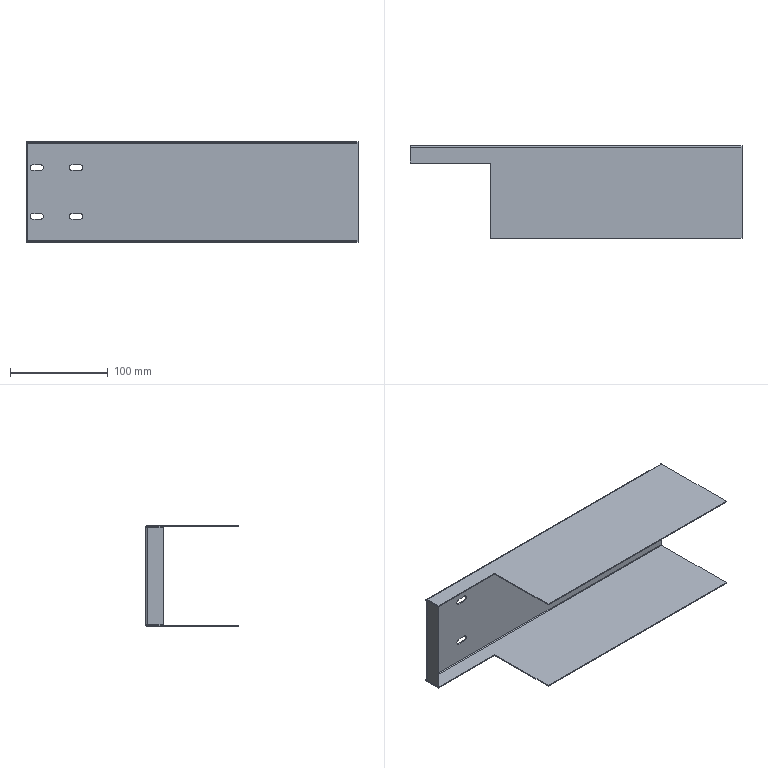Part | SolidWorks | features EdgeFlange 1, Extrusion 1, FlatPattern 1, HoleWzd 1, ICE 1, SheetMetal 1, SolidToSheetMetal 1 | 1 solid | 52 faces | box 340 x 95 x 103 mm | volume 87299 mm3 | plane 38 | cylinder 14 | commonest cylinder face diameters 5.8 x8 1.473 x3 3.473 x3
STEP:
#1=CARTESIAN_POINT('',(-163.,47.5,-27.9));
#2=VERTEX_POINT('',#1);
#3=CARTESIAN_POINT('',(-163.,47.5,-22.1));
#4=VERTEX_POINT('',#3);
#5=CARTESIAN_POINT('',(-163.,47.5,-25.));
#6=DIRECTION('',(0.,1.,0.));
#7=DIRECTION('',(0.,0.,1.));
#8=AXIS2_PLACEMENT_3D('',#5,#6,#7);
#9=CIRCLE('',#8,2.9);
#10=EDGE_CURVE('',#2,#4,#9,.T.);
#11=ORIENTED_EDGE('',*,*,#10,.F.);
#12=CARTESIAN_POINT('',(-155.,47.5,-27.9));
#13=VERTEX_POINT('',#12);
#14=CARTESIAN_POINT('',(-163.,47.5,-27.9));
#15=DIRECTION('',(1.,0.,0.));
#16=VECTOR('',#15,1000.);
#17=LINE('',#14,#16);
#18=EDGE_CURVE('',#2,#13,#17,.T.);
#19=ORIENTED_EDGE('',*,*,#18,.T.);
#20=CARTESIAN_POINT('',(-155.,47.5,-22.1));
#21=VERTEX_POINT('',#20);
#22=CARTESIAN_POINT('',(-155.,47.5,-25.));
#23=DIRECTION('',(0.,1.,0.));
#24=DIRECTION('',(0.,0.,1.));
#25=AXIS2_PLACEMENT_3D('',#22,#23,#24);
#26=CIRCLE('',#25,2.9);
#27=EDGE_CURVE('',#21,#13,#26,.T.);
#28=ORIENTED_EDGE('',*,*,#27,.F.);
#29=CARTESIAN_POINT('',(-163.,47.5,-22.1));
#30=DIRECTION('',(1.,0.,0.));
#31=VECTOR('',#30,1000.);
#32=LINE('',#29,#31);
#33=EDGE_CURVE('',#4,#21,#32,.T.);
#34=ORIENTED_EDGE('',*,*,#33,.F.);
#35=EDGE_LOOP('',(#11,#19,#28,#34));
#36=FACE_BOUND('',#35,.T.);
#37=CARTESIAN_POINT('',(-123.,47.5,-27.9));
#38=VERTEX_POINT('',#37);
#39=CARTESIAN_POINT('',(-123.,47.5,-22.1));
#40=VERTEX_POINT('',#39);
#41=CARTESIAN_POINT('',(-123.,47.5,-25.));
#42=DIRECTION('',(0.,1.,0.));
#43=DIRECTION('',(0.,0.,1.));
#44=AXIS2_PLACEMENT_3D('',#41,#42,#43);
#45=CIRCLE('',#44,2.9);
#46=EDGE_CURVE('',#38,#40,#45,.T.);
#47=ORIENTED_EDGE('',*,*,#46,.F.);
#48=CARTESIAN_POINT('',(-115.,47.5,-27.9));
#49=VERTEX_POINT('',#48);
#50=CARTESIAN_POINT('',(-123.,47.5,-27.9));
#51=DIRECTION('',(1.,0.,0.));
#52=VECTOR('',#51,1000.);
#53=LINE('',#50,#52);
#54=EDGE_CURVE('',#38,#49,#53,.T.);
#55=ORIENTED_EDGE('',*,*,#54,.T.);
#56=CARTESIAN_POINT('',(-115.,47.5,-22.1));
#57=VERTEX_POINT('',#56);
#58=CARTESIAN_POINT('',(-115.,47.5,-25.));
#59=DIRECTION('',(0.,1.,0.));
#60=DIRECTION('',(0.,0.,1.));
#61=AXIS2_PLACEMENT_3D('',#58,#59,#60);
#62=CIRCLE('',#61,2.9);
#63=EDGE_CURVE('',#57,#49,#62,.T.);
#64=ORIENTED_EDGE('',*,*,#63,.F.);
#65=CARTESIAN_POINT('',(-123.,47.5,-22.1));
#66=DIRECTION('',(1.,0.,0.));
#67=VECTOR('',#66,1000.);
#68=LINE('',#65,#67);
#69=EDGE_CURVE('',#40,#57,#68,.T.);
#70=ORIENTED_EDGE('',*,*,#69,.F.);
#71=EDGE_LOOP('',(#47,#55,#64,#70));
#72=FACE_BOUND('',#71,.T.);
#73=CARTESIAN_POINT('',(-168.263,47.5,-49.763));
#74=VERTEX_POINT('',#73);
#75=CARTESIAN_POINT('',(-168.263,47.5,49.763));
#76=VERTEX_POINT('',#75);
#77=CARTESIAN_POINT('',(-168.263,47.5,-49.763));
#78=DIRECTION('',(0.,0.,1.));
#79=VECTOR('',#78,1000.);
#80=LINE('',#77,#79);
#81=EDGE_CURVE('',#74,#76,#80,.T.);
#82=ORIENTED_EDGE('',*,*,#81,.T.);
#83=CARTESIAN_POINT('',(170.,47.5,49.763));
#84=VERTEX_POINT('',#83);
#85=CARTESIAN_POINT('',(-170.,47.5,49.763));
#86=DIRECTION('',(1.,0.,0.));
#87=VECTOR('',#86,1000.);
#88=LINE('',#85,#87);
#89=EDGE_CURVE('',#76,#84,#88,.T.);
#90=ORIENTED_EDGE('',*,*,#89,.T.);
#91=CARTESIAN_POINT('',(170.,47.5,-49.763));
#92=VERTEX_POINT('',#91);
#93=CARTESIAN_POINT('',(170.,47.5,51.5));
#94=DIRECTION('',(0.,0.,-1.));
#95=VECTOR('',#94,1000.);
#96=LINE('',#93,#95);
#97=EDGE_CURVE('',#84,#92,#96,.T.);
#98=ORIENTED_EDGE('',*,*,#97,.T.);
#99=CARTESIAN_POINT('',(-170.,47.5,-49.763));
#100=DIRECTION('',(-1.,0.,0.));
#101=VECTOR('',#100,1000.);
#102=LINE('',#99,#101);
#103=EDGE_CURVE('',#92,#74,#102,.T.);
#104=ORIENTED_EDGE('',*,*,#103,.T.);
#105=EDGE_LOOP('',(#82,#90,#98,#104));
#106=FACE_OUTER_BOUND('',#105,.T.);
#107=CARTESIAN_POINT('',(-123.,47.5,22.1));
#108=VERTEX_POINT('',#107);
#109=CARTESIAN_POINT('',(-123.,47.5,27.9));
#110=VERTEX_POINT('',#109);
#111=CARTESIAN_POINT('',(-123.,47.5,25.));
#112=DIRECTION('',(0.,1.,0.));
#113=DIRECTION('',(0.,0.,1.));
#114=AXIS2_PLACEMENT_3D('',#111,#112,#113);
#115=CIRCLE('',#114,2.9);
#116=EDGE_CURVE('',#108,#110,#115,.T.);
#117=ORIENTED_EDGE('',*,*,#116,.F.);
#118=CARTESIAN_POINT('',(-115.,47.5,22.1));
#119=VERTEX_POINT('',#118);
#120=CARTESIAN_POINT('',(-123.,47.5,22.1));
#121=DIRECTION('',(1.,0.,0.));
#122=VECTOR('',#121,1000.);
#123=LINE('',#120,#122);
#124=EDGE_CURVE('',#108,#119,#123,.T.);
#125=ORIENTED_EDGE('',*,*,#124,.T.);
#126=CARTESIAN_POINT('',(-115.,47.5,27.9));
#127=VERTEX_POINT('',#126);
#128=CARTESIAN_POINT('',(-115.,47.5,25.));
#129=DIRECTION('',(0.,1.,0.));
#130=DIRECTION('',(0.,0.,1.));
#131=AXIS2_PLACEMENT_3D('',#128,#129,#130);
#132=CIRCLE('',#131,2.9);
#133=EDGE_CURVE('',#127,#119,#132,.T.);
#134=ORIENTED_EDGE('',*,*,#133,.F.);
#135=CARTESIAN_POINT('',(-123.,47.5,27.9));
#136=DIRECTION('',(1.,0.,0.));
#137=VECTOR('',#136,1000.);
#138=LINE('',#135,#137);
#139=EDGE_CURVE('',#110,#127,#138,.T.);
#140=ORIENTED_EDGE('',*,*,#139,.F.);
#141=EDGE_LOOP('',(#117,#125,#134,#140));
#142=FACE_BOUND('',#141,.T.);
#143=CARTESIAN_POINT('',(-163.,47.5,27.9));
#144=VERTEX_POINT('',#143);
#145=CARTESIAN_POINT('',(-155.,47.5,27.9));
#146=VERTEX_POINT('',#145);
#147=CARTESIAN_POINT('',(-163.,47.5,27.9));
#148=DIRECTION('',(1.,0.,0.));
#149=VECTOR('',#148,1000.);
#150=LINE('',#147,#149);
#151=EDGE_CURVE('',#144,#146,#150,.T.);
#152=ORIENTED_EDGE('',*,*,#151,.F.);
#153=CARTESIAN_POINT('',(-163.,47.5,22.1));
#154=VERTEX_POINT('',#153);
#155=CARTESIAN_POINT('',(-163.,47.5,25.));
#156=DIRECTION('',(0.,1.,0.));
#157=DIRECTION('',(0.,0.,1.));
#158=AXIS2_PLACEMENT_3D('',#155,#156,#157);
#159=CIRCLE('',#158,2.9);
#160=EDGE_CURVE('',#154,#144,#159,.T.);
#161=ORIENTED_EDGE('',*,*,#160,.F.);
#162=CARTESIAN_POINT('',(-155.,47.5,22.1));
#163=VERTEX_POINT('',#162);
#164=CARTESIAN_POINT('',(-163.,47.5,22.1));
#165=DIRECTION('',(1.,0.,0.));
#166=VECTOR('',#165,1000.);
#167=LINE('',#164,#166);
#168=EDGE_CURVE('',#154,#163,#167,.T.);
#169=ORIENTED_EDGE('',*,*,#168,.T.);
#170=CARTESIAN_POINT('',(-155.,47.5,25.));
#171=DIRECTION('',(0.,1.,0.));
#172=DIRECTION('',(0.,0.,1.));
#173=AXIS2_PLACEMENT_3D('',#170,#171,#172);
#174=CIRCLE('',#173,2.9);
#175=EDGE_CURVE('',#146,#163,#174,.T.);
#176=ORIENTED_EDGE('',*,*,#175,.F.);
#177=EDGE_LOOP('',(#152,#161,#169,#176));
#178=FACE_BOUND('',#177,.T.);
#179=CARTESIAN_POINT('',(-170.,47.5,51.5));
#180=DIRECTION('',(0.,-1.,0.));
#181=DIRECTION('',(0.,0.,-1.));
#182=AXIS2_PLACEMENT_3D('',#179,#180,#181);
#183=PLANE('',#182);
#184=ADVANCED_FACE('',(#36,#72,#106,#142,#178),#183,.F.);
#185=CARTESIAN_POINT('',(-170.,47.5,49.763));
#186=VERTEX_POINT('',#185);
#187=CARTESIAN_POINT('',(-170.,47.5,49.763));
#188=DIRECTION('',(1.,0.,0.));
#189=VECTOR('',#188,1000.);
#190=LINE('',#187,#189);
#191=EDGE_CURVE('',#186,#76,#190,.T.);
#192=ORIENTED_EDGE('',*,*,#191,.T.);
#193=CARTESIAN_POINT('',(-169.836,46.5,49.763));
#194=VERTEX_POINT('',#193);
#195=CARTESIAN_POINT('',(-168.263,45.763,49.763));
#196=DIRECTION('',(0.,0.,1.));
#197=DIRECTION('',(-1.,0.,0.));
#198=AXIS2_PLACEMENT_3D('',#195,#196,#197);
#199=CIRCLE('',#198,1.737);
#200=EDGE_CURVE('',#76,#194,#199,.T.);
#201=ORIENTED_EDGE('',*,*,#200,.T.);
#202=CARTESIAN_POINT('',(-170.,46.5,49.763));
#203=VERTEX_POINT('',#202);
#204=CARTESIAN_POINT('',(-170.,46.5,49.763));
#205=DIRECTION('',(1.,0.,0.));
#206=VECTOR('',#205,1000.);
#207=LINE('',#204,#206);
#208=EDGE_CURVE('',#203,#194,#207,.T.);
#209=ORIENTED_EDGE('',*,*,#208,.F.);
#210=CARTESIAN_POINT('',(-170.,47.5,49.763));
#211=DIRECTION('',(0.,1.,0.));
#212=VECTOR('',#211,1000.);
#213=LINE('',#210,#212);
#214=EDGE_CURVE('',#203,#186,#213,.T.);
#215=ORIENTED_EDGE('',*,*,#214,.T.);
#216=EDGE_LOOP('',(#192,#201,#209,#215));
#217=FACE_OUTER_BOUND('',#216,.T.);
#218=CARTESIAN_POINT('',(-168.263,46.5,49.763));
#219=DIRECTION('',(0.,0.,-1.));
#220=DIRECTION('',(0.,1.,0.));
#221=AXIS2_PLACEMENT_3D('',#218,#219,#220);
#222=PLANE('',#221);
#223=ADVANCED_FACE('',(#217),#222,.T.);
#224=CARTESIAN_POINT('',(-170.,46.5,-49.763));
#225=VERTEX_POINT('',#224);
#226=CARTESIAN_POINT('',(-169.836,46.5,-49.763));
#227=VERTEX_POINT('',#226);
#228=CARTESIAN_POINT('',(-170.,46.5,-49.763));
#229=DIRECTION('',(1.,0.,0.));
#230=VECTOR('',#229,1000.);
#231=LINE('',#228,#230);
#232=EDGE_CURVE('',#225,#227,#231,.T.);
#233=ORIENTED_EDGE('',*,*,#232,.T.);
#234=CARTESIAN_POINT('',(-168.263,45.763,-49.763));
#235=DIRECTION('',(0.,0.,-1.));
#236=DIRECTION('',(-1.,0.,0.));
#237=AXIS2_PLACEMENT_3D('',#234,#235,#236);
#238=CIRCLE('',#237,1.737);
#239=EDGE_CURVE('',#227,#74,#238,.T.);
#240=ORIENTED_EDGE('',*,*,#239,.T.);
#241=CARTESIAN_POINT('',(-170.,47.5,-49.763));
#242=VERTEX_POINT('',#241);
#243=CARTESIAN_POINT('',(-170.,47.5,-49.763));
#244=DIRECTION('',(1.,0.,0.));
#245=VECTOR('',#244,1000.);
#246=LINE('',#243,#245);
#247=EDGE_CURVE('',#242,#74,#246,.T.);
#248=ORIENTED_EDGE('',*,*,#247,.F.);
#249=CARTESIAN_POINT('',(-170.,47.5,-49.763));
#250=DIRECTION('',(0.,1.,0.));
#251=VECTOR('',#250,1000.);
#252=LINE('',#249,#251);
#253=EDGE_CURVE('',#225,#242,#252,.T.);
#254=ORIENTED_EDGE('',*,*,#253,.F.);
#255=EDGE_LOOP('',(#233,#240,#248,#254));
#256=FACE_OUTER_BOUND('',#255,.T.);
#257=CARTESIAN_POINT('',(-170.,46.5,-49.763));
#258=DIRECTION('',(0.,0.,1.));
#259=DIRECTION('',(1.,0.,0.));
#260=AXIS2_PLACEMENT_3D('',#257,#258,#259);
#261=PLANE('',#260);
#262=ADVANCED_FACE('',(#256),#261,.T.);
#263=CARTESIAN_POINT('',(-163.,46.5,-27.9));
#264=VERTEX_POINT('',#263);
#265=CARTESIAN_POINT('',(-155.,46.5,-27.9));
#266=VERTEX_POINT('',#265);
#267=CARTESIAN_POINT('',(-170.,46.5,-27.9));
#268=DIRECTION('',(1.,0.,0.));
#269=VECTOR('',#268,1000.);
#270=LINE('',#267,#269);
#271=EDGE_CURVE('',#264,#266,#270,.T.);
#272=ORIENTED_EDGE('',*,*,#271,.F.);
#273=CARTESIAN_POINT('',(-163.,46.5,-22.1));
#274=VERTEX_POINT('',#273);
#275=CARTESIAN_POINT('',(-163.,46.5,-25.));
#276=DIRECTION('',(0.,-1.,0.));
#277=DIRECTION('',(0.,0.,-1.));
#278=AXIS2_PLACEMENT_3D('',#275,#276,#277);
#279=CIRCLE('',#278,2.9);
#280=EDGE_CURVE('',#274,#264,#279,.T.);
#281=ORIENTED_EDGE('',*,*,#280,.F.);
#282=CARTESIAN_POINT('',(-155.,46.5,-22.1));
#283=VERTEX_POINT('',#282);
#284=CARTESIAN_POINT('',(-170.,46.5,-22.1));
#285=DIRECTION('',(-1.,0.,0.));
#286=VECTOR('',#285,1000.);
#287=LINE('',#284,#286);
#288=EDGE_CURVE('',#283,#274,#287,.T.);
#289=ORIENTED_EDGE('',*,*,#288,.F.);
#290=CARTESIAN_POINT('',(-155.,46.5,-25.));
#291=DIRECTION('',(0.,-1.,0.));
#292=DIRECTION('',(0.,0.,-1.));
#293=AXIS2_PLACEMENT_3D('',#290,#291,#292);
#294=CIRCLE('',#293,2.9);
#295=EDGE_CURVE('',#266,#283,#294,.T.);
#296=ORIENTED_EDGE('',*,*,#295,.F.);
#297=EDGE_LOOP('',(#272,#281,#289,#296));
#298=FACE_BOUND('',#297,.T.);
#299=CARTESIAN_POINT('',(-123.,46.5,-27.9));
#300=VERTEX_POINT('',#299);
#301=CARTESIAN_POINT('',(-115.,46.5,-27.9));
#302=VERTEX_POINT('',#301);
#303=CARTESIAN_POINT('',(-170.,46.5,-27.9));
#304=DIRECTION('',(1.,0.,0.));
#305=VECTOR('',#304,1000.);
#306=LINE('',#303,#305);
#307=EDGE_CURVE('',#300,#302,#306,.T.);
#308=ORIENTED_EDGE('',*,*,#307,.F.);
#309=CARTESIAN_POINT('',(-123.,46.5,-22.1));
#310=VERTEX_POINT('',#309);
#311=CARTESIAN_POINT('',(-123.,46.5,-25.));
#312=DIRECTION('',(0.,-1.,0.));
#313=DIRECTION('',(0.,0.,-1.));
#314=AXIS2_PLACEMENT_3D('',#311,#312,#313);
#315=CIRCLE('',#314,2.9);
#316=EDGE_CURVE('',#310,#300,#315,.T.);
#317=ORIENTED_EDGE('',*,*,#316,.F.);
#318=CARTESIAN_POINT('',(-115.,46.5,-22.1));
#319=VERTEX_POINT('',#318);
#320=CARTESIAN_POINT('',(-170.,46.5,-22.1));
#321=DIRECTION('',(-1.,0.,0.));
#322=VECTOR('',#321,1000.);
#323=LINE('',#320,#322);
#324=EDGE_CURVE('',#319,#310,#323,.T.);
#325=ORIENTED_EDGE('',*,*,#324,.F.);
#326=CARTESIAN_POINT('',(-115.,46.5,-25.));
#327=DIRECTION('',(0.,-1.,0.));
#328=DIRECTION('',(0.,0.,-1.));
#329=AXIS2_PLACEMENT_3D('',#326,#327,#328);
#330=CIRCLE('',#329,2.9);
#331=EDGE_CURVE('',#302,#319,#330,.T.);
#332=ORIENTED_EDGE('',*,*,#331,.F.);
#333=EDGE_LOOP('',(#308,#317,#325,#332));
#334=FACE_BOUND('',#333,.T.);
#335=CARTESIAN_POINT('',(-155.,46.5,22.1));
#336=VERTEX_POINT('',#335);
#337=CARTESIAN_POINT('',(-155.,46.5,27.9));
#338=VERTEX_POINT('',#337);
#339=CARTESIAN_POINT('',(-155.,46.5,25.));
#340=DIRECTION('',(0.,-1.,0.));
#341=DIRECTION('',(0.,0.,-1.));
#342=AXIS2_PLACEMENT_3D('',#339,#340,#341);
#343=CIRCLE('',#342,2.9);
#344=EDGE_CURVE('',#336,#338,#343,.T.);
#345=ORIENTED_EDGE('',*,*,#344,.F.);
#346=CARTESIAN_POINT('',(-163.,46.5,22.1));
#347=VERTEX_POINT('',#346);
#348=CARTESIAN_POINT('',(-170.,46.5,22.1));
#349=DIRECTION('',(1.,0.,0.));
#350=VECTOR('',#349,1000.);
#351=LINE('',#348,#350);
#352=EDGE_CURVE('',#347,#336,#351,.T.);
#353=ORIENTED_EDGE('',*,*,#352,.F.);
#354=CARTESIAN_POINT('',(-163.,46.5,27.9));
#355=VERTEX_POINT('',#354);
#356=CARTESIAN_POINT('',(-163.,46.5,25.));
#357=DIRECTION('',(0.,-1.,0.));
#358=DIRECTION('',(0.,0.,-1.));
#359=AXIS2_PLACEMENT_3D('',#356,#357,#358);
#360=CIRCLE('',#359,2.9);
#361=EDGE_CURVE('',#355,#347,#360,.T.);
#362=ORIENTED_EDGE('',*,*,#361,.F.);
#363=CARTESIAN_POINT('',(-170.,46.5,27.9));
#364=DIRECTION('',(-1.,0.,0.));
#365=VECTOR('',#364,1000.);
#366=LINE('',#363,#365);
#367=EDGE_CURVE('',#338,#355,#366,.T.);
#368=ORIENTED_EDGE('',*,*,#367,.F.);
#369=EDGE_LOOP('',(#345,#353,#362,#368));
#370=FACE_BOUND('',#369,.T.);
#371=CARTESIAN_POINT('',(-123.,46.5,22.1));
#372=VERTEX_POINT('',#371);
#373=CARTESIAN_POINT('',(-115.,46.5,22.1));
#374=VERTEX_POINT('',#373);
#375=CARTESIAN_POINT('',(-170.,46.5,22.1));
#376=DIRECTION('',(1.,0.,0.));
#377=VECTOR('',#376,1000.);
#378=LINE('',#375,#377);
#379=EDGE_CURVE('',#372,#374,#378,.T.);
#380=ORIENTED_EDGE('',*,*,#379,.F.);
#381=CARTESIAN_POINT('',(-123.,46.5,27.9));
#382=VERTEX_POINT('',#381);
#383=CARTESIAN_POINT('',(-123.,46.5,25.));
#384=DIRECTION('',(0.,-1.,0.));
#385=DIRECTION('',(0.,0.,-1.));
#386=AXIS2_PLACEMENT_3D('',#383,#384,#385);
#387=CIRCLE('',#386,2.9);
#388=EDGE_CURVE('',#382,#372,#387,.T.);
#389=ORIENTED_EDGE('',*,*,#388,.F.);
#390=CARTESIAN_POINT('',(-115.,46.5,27.9));
#391=VERTEX_POINT('',#390);
#392=CARTESIAN_POINT('',(-170.,46.5,27.9));
#393=DIRECTION('',(-1.,0.,0.));
#394=VECTOR('',#393,1000.);
#395=LINE('',#392,#394);
#396=EDGE_CURVE('',#391,#382,#395,.T.);
#397=ORIENTED_EDGE('',*,*,#396,.F.);
#398=CARTESIAN_POINT('',(-115.,46.5,25.));
#399=DIRECTION('',(0.,-1.,0.));
#400=DIRECTION('',(0.,0.,-1.));
#401=AXIS2_PLACEMENT_3D('',#398,#399,#400);
#402=CIRCLE('',#401,2.9);
#403=EDGE_CURVE('',#374,#391,#402,.T.);
#404=ORIENTED_EDGE('',*,*,#403,.F.);
#405=EDGE_LOOP('',(#380,#389,#397,#404));
#406=FACE_BOUND('',#405,.T.);
#407=CARTESIAN_POINT('',(-168.263,46.5,49.763));
#408=VERTEX_POINT('',#407);
#409=CARTESIAN_POINT('',(170.,46.5,49.763));
#410=VERTEX_POINT('',#409);
#411=CARTESIAN_POINT('',(-170.,46.5,49.763));
#412=DIRECTION('',(1.,0.,0.));
#413=VECTOR('',#412,1000.);
#414=LINE('',#411,#413);
#415=EDGE_CURVE('',#408,#410,#414,.T.);
#416=ORIENTED_EDGE('',*,*,#415,.F.);
#417=CARTESIAN_POINT('',(-168.263,46.5,-49.763));
#418=VERTEX_POINT('',#417);
#419=CARTESIAN_POINT('',(-168.263,46.5,-49.763));
#420=DIRECTION('',(0.,0.,1.));
#421=VECTOR('',#420,1000.);
#422=LINE('',#419,#421);
#423=EDGE_CURVE('',#418,#408,#422,.T.);
#424=ORIENTED_EDGE('',*,*,#423,.F.);
#425=CARTESIAN_POINT('',(170.,46.5,-49.763));
#426=VERTEX_POINT('',#425);
#427=CARTESIAN_POINT('',(-170.,46.5,-49.763));
#428=DIRECTION('',(-1.,0.,0.));
#429=VECTOR('',#428,1000.);
#430=LINE('',#427,#429);
#431=EDGE_CURVE('',#426,#418,#430,.T.);
#432=ORIENTED_EDGE('',*,*,#431,.F.);
#433=CARTESIAN_POINT('',(170.,46.5,51.5));
#434=DIRECTION('',(0.,0.,-1.));
#435=VECTOR('',#434,1000.);
#436=LINE('',#433,#435);
#437=EDGE_CURVE('',#410,#426,#436,.T.);
#438=ORIENTED_EDGE('',*,*,#437,.F.);
#439=EDGE_LOOP('',(#416,#424,#432,#438));
#440=FACE_OUTER_BOUND('',#439,.T.);
#441=CARTESIAN_POINT('',(-170.,46.5,51.5));
#442=DIRECTION('',(0.,-1.,0.));
#443=DIRECTION('',(0.,0.,-1.));
#444=AXIS2_PLACEMENT_3D('',#441,#442,#443);
#445=PLANE('',#444);
#446=ADVANCED_FACE('',(#298,#334,#370,#406,#440),#445,.T.);
#447=CARTESIAN_POINT('',(170.,47.5,49.763));
#448=DIRECTION('',(0.,1.,0.));
#449=VECTOR('',#448,1000.);
#450=LINE('',#447,#449);
#451=EDGE_CURVE('',#410,#84,#450,.T.);
#452=ORIENTED_EDGE('',*,*,#451,.F.);
#453=ORIENTED_EDGE('',*,*,#437,.T.);
#454=CARTESIAN_POINT('',(170.,47.5,-49.763));
#455=DIRECTION('',(0.,1.,0.));
#456=VECTOR('',#455,1000.);
#457=LINE('',#454,#456);
#458=EDGE_CURVE('',#426,#92,#457,.T.);
#459=ORIENTED_EDGE('',*,*,#458,.T.);
#460=ORIENTED_EDGE('',*,*,#97,.F.);
#461=EDGE_LOOP('',(#452,#453,#459,#460));
#462=FACE_OUTER_BOUND('',#461,.T.);
#463=CARTESIAN_POINT('',(170.,47.5,51.5));
#464=DIRECTION('',(-1.,0.,0.));
#465=DIRECTION('',(0.,0.,-1.));
#466=AXIS2_PLACEMENT_3D('',#463,#464,#465);
#467=PLANE('',#466);
#468=ADVANCED_FACE('',(#462),#467,.F.);
#469=ORIENTED_EDGE('',*,*,#458,.F.);
#470=CARTESIAN_POINT('',(170.,45.763,-50.5));
#471=VERTEX_POINT('',#470);
#472=CARTESIAN_POINT('',(170.,45.763,-49.763));
#473=DIRECTION('',(-1.,0.,0.));
#474=DIRECTION('',(0.,0.,-1.));
#475=AXIS2_PLACEMENT_3D('',#472,#473,#474);
#476=CIRCLE('',#475,0.7366);
#477=EDGE_CURVE('',#426,#471,#476,.T.);
#478=ORIENTED_EDGE('',*,*,#477,.T.);
#479=CARTESIAN_POINT('',(170.,45.763,-51.5));
#480=VERTEX_POINT('',#479);
#481=CARTESIAN_POINT('',(170.,45.763,-51.5));
#482=DIRECTION('',(0.,0.,-1.));
#483=VECTOR('',#482,1000.);
#484=LINE('',#481,#483);
#485=EDGE_CURVE('',#471,#480,#484,.T.);
#486=ORIENTED_EDGE('',*,*,#485,.T.);
#487=CARTESIAN_POINT('',(170.,45.763,-49.763));
#488=DIRECTION('',(-1.,0.,0.));
#489=DIRECTION('',(0.,0.,1.));
#490=AXIS2_PLACEMENT_3D('',#487,#488,#489);
#491=CIRCLE('',#490,1.737);
#492=EDGE_CURVE('',#92,#480,#491,.T.);
#493=ORIENTED_EDGE('',*,*,#492,.F.);
#494=EDGE_LOOP('',(#469,#478,#486,#493));
#495=FACE_OUTER_BOUND('',#494,.T.);
#496=CARTESIAN_POINT('',(170.,45.763,-49.763));
#497=DIRECTION('',(1.,0.,0.));
#498=DIRECTION('',(0.,0.,-1.));
#499=AXIS2_PLACEMENT_3D('',#496,#497,#498);
#500=PLANE('',#499);
#501=ADVANCED_FACE('',(#495),#500,.T.);
#502=ORIENTED_EDGE('',*,*,#485,.F.);
#503=CARTESIAN_POINT('',(170.,-47.5,-50.5));
#504=VERTEX_POINT('',#503);
#505=CARTESIAN_POINT('',(170.,0.,-50.5));
#506=DIRECTION('',(0.,1.,0.));
#507=VECTOR('',#506,1000.);
#508=LINE('',#505,#507);
#509=EDGE_CURVE('',#504,#471,#508,.T.);
#510=ORIENTED_EDGE('',*,*,#509,.F.);
#511=CARTESIAN_POINT('',(170.,-47.5,-51.5));
#512=VERTEX_POINT('',#511);
#513=CARTESIAN_POINT('',(170.,-47.5,-51.5));
#514=DIRECTION('',(0.,0.,-1.));
#515=VECTOR('',#514,1000.);
#516=LINE('',#513,#515);
#517=EDGE_CURVE('',#504,#512,#516,.T.);
#518=ORIENTED_EDGE('',*,*,#517,.T.);
#519=CARTESIAN_POINT('',(170.,-47.5,-51.5));
#520=DIRECTION('',(0.,1.,0.));
#521=VECTOR('',#520,1000.);
#522=LINE('',#519,#521);
#523=EDGE_CURVE('',#512,#480,#522,.T.);
#524=ORIENTED_EDGE('',*,*,#523,.T.);
#525=EDGE_LOOP('',(#502,#510,#518,#524));
#526=FACE_OUTER_BOUND('',#525,.T.);
#527=CARTESIAN_POINT('',(170.,-47.5,-51.5));
#528=DIRECTION('',(-1.,0.,0.));
#529=DIRECTION('',(0.,1.,0.));
#530=AXIS2_PLACEMENT_3D('',#527,#528,#529);
#531=PLANE('',#530);
#532=ADVANCED_FACE('',(#526),#531,.F.);
#533=CARTESIAN_POINT('',(-88.,-47.5,-50.5));
#534=VERTEX_POINT('',#533);
#535=CARTESIAN_POINT('',(-88.,-47.5,-51.5));
#536=VERTEX_POINT('',#535);
#537=CARTESIAN_POINT('',(-88.,-47.5,51.5));
#538=DIRECTION('',(0.,0.,-1.));
#539=VECTOR('',#538,1000.);
#540=LINE('',#537,#539);
#541=EDGE_CURVE('',#534,#536,#540,.T.);
#542=ORIENTED_EDGE('',*,*,#541,.T.);
#543=CARTESIAN_POINT('',(-170.,-47.5,-51.5));
#544=DIRECTION('',(1.,0.,0.));
#545=VECTOR('',#544,1000.);
#546=LINE('',#543,#545);
#547=EDGE_CURVE('',#536,#512,#546,.T.);
#548=ORIENTED_EDGE('',*,*,#547,.T.);
#549=ORIENTED_EDGE('',*,*,#517,.F.);
#550=CARTESIAN_POINT('',(0.,-47.5,-50.5));
#551=DIRECTION('',(1.,0.,0.));
#552=VECTOR('',#551,1000.);
#553=LINE('',#550,#552);
#554=EDGE_CURVE('',#534,#504,#553,.T.);
#555=ORIENTED_EDGE('',*,*,#554,.F.);
#556=EDGE_LOOP('',(#542,#548,#549,#555));
#557=FACE_OUTER_BOUND('',#556,.T.);
#558=CARTESIAN_POINT('',(-170.,-47.5,-51.5));
#559=DIRECTION('',(0.,1.,0.));
#560=DIRECTION('',(1.,0.,0.));
#561=AXIS2_PLACEMENT_3D('',#558,#559,#560);
#562=PLANE('',#561);
#563=ADVANCED_FACE('',(#557),#562,.F.);
#564=CARTESIAN_POINT('',(-170.,29.5,-50.5));
#565=VERTEX_POINT('',#564);
#566=CARTESIAN_POINT('',(-170.,29.5,-51.5));
#567=VERTEX_POINT('',#566);
#568=CARTESIAN_POINT('',(-170.,29.5,51.5));
#569=DIRECTION('',(0.,0.,-1.));
#570=VECTOR('',#569,1000.);
#571=LINE('',#568,#570);
#572=EDGE_CURVE('',#565,#567,#571,.T.);
#573=ORIENTED_EDGE('',*,*,#572,.F.);
#574=CARTESIAN_POINT('',(-170.,45.763,-50.5));
#575=VERTEX_POINT('',#574);
#576=CARTESIAN_POINT('',(-170.,0.,-50.5));
#577=DIRECTION('',(0.,-1.,0.));
#578=VECTOR('',#577,1000.);
#579=LINE('',#576,#578);
#580=EDGE_CURVE('',#575,#565,#579,.T.);
#581=ORIENTED_EDGE('',*,*,#580,.F.);
#582=CARTESIAN_POINT('',(-170.,45.763,-51.5));
#583=VERTEX_POINT('',#582);
#584=CARTESIAN_POINT('',(-170.,45.763,-51.5));
#585=DIRECTION('',(0.,0.,-1.));
#586=VECTOR('',#585,1000.);
#587=LINE('',#584,#586);
#588=EDGE_CURVE('',#575,#583,#587,.T.);
#589=ORIENTED_EDGE('',*,*,#588,.T.);
#590=CARTESIAN_POINT('',(-170.,-47.5,-51.5));
#591=DIRECTION('',(0.,-1.,0.));
#592=VECTOR('',#591,1000.);
#593=LINE('',#590,#592);
#594=EDGE_CURVE('',#583,#567,#593,.T.);
#595=ORIENTED_EDGE('',*,*,#594,.T.);
#596=EDGE_LOOP('',(#573,#581,#589,#595));
#597=FACE_OUTER_BOUND('',#596,.T.);
#598=CARTESIAN_POINT('',(-170.,-47.5,-51.5));
#599=DIRECTION('',(1.,0.,0.));
#600=DIRECTION('',(0.,-1.,0.));
#601=AXIS2_PLACEMENT_3D('',#598,#599,#600);
#602=PLANE('',#601);
#603=ADVANCED_FACE('',(#597),#602,.F.);
#604=ORIENTED_EDGE('',*,*,#588,.F.);
#605=CARTESIAN_POINT('',(-170.,45.763,-49.763));
#606=DIRECTION('',(1.,0.,0.));
#607=DIRECTION('',(0.,0.,-1.));
#608=AXIS2_PLACEMENT_3D('',#605,#606,#607);
#609=CIRCLE('',#608,0.7366);
#610=EDGE_CURVE('',#575,#225,#609,.T.);
#611=ORIENTED_EDGE('',*,*,#610,.T.);
#612=ORIENTED_EDGE('',*,*,#253,.T.);
#613=CARTESIAN_POINT('',(-170.,45.763,-49.763));
#614=DIRECTION('',(1.,0.,0.));
#615=DIRECTION('',(0.,0.,1.));
#616=AXIS2_PLACEMENT_3D('',#613,#614,#615);
#617=CIRCLE('',#616,1.737);
#618=EDGE_CURVE('',#583,#242,#617,.T.);
#619=ORIENTED_EDGE('',*,*,#618,.F.);
#620=EDGE_LOOP('',(#604,#611,#612,#619));
#621=FACE_OUTER_BOUND('',#620,.T.);
#622=CARTESIAN_POINT('',(-170.,45.763,-49.763));
#623=DIRECTION('',(1.,0.,0.));
#624=DIRECTION('',(0.,0.,-1.));
#625=AXIS2_PLACEMENT_3D('',#622,#623,#624);
#626=PLANE('',#625);
#627=ADVANCED_FACE('',(#621),#626,.F.);
#628=ORIENTED_EDGE('',*,*,#214,.F.);
#629=CARTESIAN_POINT('',(-170.,45.763,50.5));
#630=VERTEX_POINT('',#629);
#631=CARTESIAN_POINT('',(-170.,45.763,49.763));
#632=DIRECTION('',(1.,0.,0.));
#633=DIRECTION('',(0.,0.,1.));
#634=AXIS2_PLACEMENT_3D('',#631,#632,#633);
#635=CIRCLE('',#634,0.7366);
#636=EDGE_CURVE('',#203,#630,#635,.T.);
#637=ORIENTED_EDGE('',*,*,#636,.T.);
#638=CARTESIAN_POINT('',(-170.,45.763,51.5));
#639=VERTEX_POINT('',#638);
#640=CARTESIAN_POINT('',(-170.,45.763,51.5));
#641=DIRECTION('',(0.,0.,1.));
#642=VECTOR('',#641,1000.);
#643=LINE('',#640,#642);
#644=EDGE_CURVE('',#630,#639,#643,.T.);
#645=ORIENTED_EDGE('',*,*,#644,.T.);
#646=CARTESIAN_POINT('',(-170.,45.763,49.763));
#647=DIRECTION('',(1.,0.,0.));
#648=DIRECTION('',(0.,0.,-1.));
#649=AXIS2_PLACEMENT_3D('',#646,#647,#648);
#650=CIRCLE('',#649,1.737);
#651=EDGE_CURVE('',#186,#639,#650,.T.);
#652=ORIENTED_EDGE('',*,*,#651,.F.);
#653=EDGE_LOOP('',(#628,#637,#645,#652));
#654=FACE_OUTER_BOUND('',#653,.T.);
#655=CARTESIAN_POINT('',(-170.,45.763,49.763));
#656=DIRECTION('',(-1.,0.,0.));
#657=DIRECTION('',(0.,0.,1.));
#658=AXIS2_PLACEMENT_3D('',#655,#656,#657);
#659=PLANE('',#658);
#660=ADVANCED_FACE('',(#654),#659,.T.);
#661=CARTESIAN_POINT('',(-170.,29.5,51.5));
#662=VERTEX_POINT('',#661);
#663=CARTESIAN_POINT('',(-170.,29.5,50.5));
#664=VERTEX_POINT('',#663);
#665=CARTESIAN_POINT('',(-170.,29.5,51.5));
#666=DIRECTION('',(0.,0.,-1.));
#667=VECTOR('',#666,1000.);
#668=LINE('',#665,#667);
#669=EDGE_CURVE('',#662,#664,#668,.T.);
#670=ORIENTED_EDGE('',*,*,#669,.F.);
#671=CARTESIAN_POINT('',(-170.,-47.5,51.5));
#672=DIRECTION('',(0.,-1.,0.));
#673=VECTOR('',#672,1000.);
#674=LINE('',#671,#673);
#675=EDGE_CURVE('',#639,#662,#674,.T.);
#676=ORIENTED_EDGE('',*,*,#675,.F.);
#677=ORIENTED_EDGE('',*,*,#644,.F.);
#678=CARTESIAN_POINT('',(-170.,0.,50.5));
#679=DIRECTION('',(0.,-1.,0.));
#680=VECTOR('',#679,1000.);
#681=LINE('',#678,#680);
#682=EDGE_CURVE('',#630,#664,#681,.T.);
#683=ORIENTED_EDGE('',*,*,#682,.T.);
#684=EDGE_LOOP('',(#670,#676,#677,#683));
#685=FACE_OUTER_BOUND('',#684,.T.);
#686=CARTESIAN_POINT('',(-170.,-47.5,51.5));
#687=DIRECTION('',(1.,0.,0.));
#688=DIRECTION('',(0.,-1.,0.));
#689=AXIS2_PLACEMENT_3D('',#686,#687,#688);
#690=PLANE('',#689);
#691=ADVANCED_FACE('',(#685),#690,.F.);
#692=CARTESIAN_POINT('',(-88.,-47.5,51.5));
#693=VERTEX_POINT('',#692);
#694=CARTESIAN_POINT('',(-88.,-47.5,50.5));
#695=VERTEX_POINT('',#694);
#696=CARTESIAN_POINT('',(-88.,-47.5,51.5));
#697=DIRECTION('',(0.,0.,-1.));
#698=VECTOR('',#697,1000.);
#699=LINE('',#696,#698);
#700=EDGE_CURVE('',#693,#695,#699,.T.);
#701=ORIENTED_EDGE('',*,*,#700,.T.);
#702=CARTESIAN_POINT('',(170.,-47.5,50.5));
#703=VERTEX_POINT('',#702);
#704=CARTESIAN_POINT('',(0.,-47.5,50.5));
#705=DIRECTION('',(1.,0.,0.));
#706=VECTOR('',#705,1000.);
#707=LINE('',#704,#706);
#708=EDGE_CURVE('',#695,#703,#707,.T.);
#709=ORIENTED_EDGE('',*,*,#708,.T.);
#710=CARTESIAN_POINT('',(170.,-47.5,51.5));
#711=VERTEX_POINT('',#710);
#712=CARTESIAN_POINT('',(170.,-47.5,51.5));
#713=DIRECTION('',(0.,0.,1.));
#714=VECTOR('',#713,1000.);
#715=LINE('',#712,#714);
#716=EDGE_CURVE('',#703,#711,#715,.T.);
#717=ORIENTED_EDGE('',*,*,#716,.T.);
#718=CARTESIAN_POINT('',(-170.,-47.5,51.5));
#719=DIRECTION('',(1.,0.,0.));
#720=VECTOR('',#719,1000.);
#721=LINE('',#718,#720);
#722=EDGE_CURVE('',#693,#711,#721,.T.);
#723=ORIENTED_EDGE('',*,*,#722,.F.);
#724=EDGE_LOOP('',(#701,#709,#717,#723));
#725=FACE_OUTER_BOUND('',#724,.T.);
#726=CARTESIAN_POINT('',(-170.,-47.5,51.5));
#727=DIRECTION('',(0.,1.,0.));
#728=DIRECTION('',(1.,0.,0.));
#729=AXIS2_PLACEMENT_3D('',#726,#727,#728);
#730=PLANE('',#729);
#731=ADVANCED_FACE('',(#725),#730,.F.);
#732=ORIENTED_EDGE('',*,*,#716,.F.);
#733=CARTESIAN_POINT('',(170.,45.763,50.5));
#734=VERTEX_POINT('',#733);
#735=CARTESIAN_POINT('',(170.,0.,50.5));
#736=DIRECTION('',(0.,1.,0.));
#737=VECTOR('',#736,1000.);
#738=LINE('',#735,#737);
#739=EDGE_CURVE('',#703,#734,#738,.T.);
#740=ORIENTED_EDGE('',*,*,#739,.T.);
#741=CARTESIAN_POINT('',(170.,45.763,51.5));
#742=VERTEX_POINT('',#741);
#743=CARTESIAN_POINT('',(170.,45.763,51.5));
#744=DIRECTION('',(0.,0.,1.));
#745=VECTOR('',#744,1000.);
#746=LINE('',#743,#745);
#747=EDGE_CURVE('',#734,#742,#746,.T.);
#748=ORIENTED_EDGE('',*,*,#747,.T.);
#749=CARTESIAN_POINT('',(170.,-47.5,51.5));
#750=DIRECTION('',(0.,1.,0.));
#751=VECTOR('',#750,1000.);
#752=LINE('',#749,#751);
#753=EDGE_CURVE('',#711,#742,#752,.T.);
#754=ORIENTED_EDGE('',*,*,#753,.F.);
#755=EDGE_LOOP('',(#732,#740,#748,#754));
#756=FACE_OUTER_BOUND('',#755,.T.);
#757=CARTESIAN_POINT('',(170.,-47.5,51.5));
#758=DIRECTION('',(-1.,0.,0.));
#759=DIRECTION('',(0.,1.,0.));
#760=AXIS2_PLACEMENT_3D('',#757,#758,#759);
#761=PLANE('',#760);
#762=ADVANCED_FACE('',(#756),#761,.F.);
#763=CARTESIAN_POINT('',(170.,45.763,49.763));
#764=DIRECTION('',(-1.,0.,0.));
#765=DIRECTION('',(0.,0.,1.));
#766=AXIS2_PLACEMENT_3D('',#763,#764,#765);
#767=CIRCLE('',#766,0.7366);
#768=EDGE_CURVE('',#734,#410,#767,.T.);
#769=ORIENTED_EDGE('',*,*,#768,.T.);
#770=ORIENTED_EDGE('',*,*,#451,.T.);
#771=CARTESIAN_POINT('',(170.,45.763,49.763));
#772=DIRECTION('',(-1.,0.,0.));
#773=DIRECTION('',(0.,0.,-1.));
#774=AXIS2_PLACEMENT_3D('',#771,#772,#773);
#775=CIRCLE('',#774,1.737);
#776=EDGE_CURVE('',#742,#84,#775,.T.);
#777=ORIENTED_EDGE('',*,*,#776,.F.);
#778=ORIENTED_EDGE('',*,*,#747,.F.);
#779=EDGE_LOOP('',(#769,#770,#777,#778));
#780=FACE_OUTER_BOUND('',#779,.T.);
#781=CARTESIAN_POINT('',(170.,45.763,49.763));
#782=DIRECTION('',(-1.,0.,0.));
#783=DIRECTION('',(0.,0.,1.));
#784=AXIS2_PLACEMENT_3D('',#781,#782,#783);
#785=PLANE('',#784);
#786=ADVANCED_FACE('',(#780),#785,.F.);
#787=CARTESIAN_POINT('',(-88.,29.5,51.5));
#788=VERTEX_POINT('',#787);
#789=CARTESIAN_POINT('',(-170.,29.5,51.5));
#790=DIRECTION('',(1.,0.,0.));
#791=VECTOR('',#790,1000.);
#792=LINE('',#789,#791);
#793=EDGE_CURVE('',#662,#788,#792,.T.);
#794=ORIENTED_EDGE('',*,*,#793,.T.);
#795=CARTESIAN_POINT('',(-88.,29.5,51.5));
#796=DIRECTION('',(0.,-1.,0.));
#797=VECTOR('',#796,1000.);
#798=LINE('',#795,#797);
#799=EDGE_CURVE('',#788,#693,#798,.T.);
#800=ORIENTED_EDGE('',*,*,#799,.T.);
#801=ORIENTED_EDGE('',*,*,#722,.T.);
#802=ORIENTED_EDGE('',*,*,#753,.T.);
#803=CARTESIAN_POINT('',(0.,45.763,51.5));
#804=DIRECTION('',(-1.,0.,0.));
#805=VECTOR('',#804,1000.);
#806=LINE('',#803,#805);
#807=EDGE_CURVE('',#742,#639,#806,.T.);
#808=ORIENTED_EDGE('',*,*,#807,.T.);
#809=ORIENTED_EDGE('',*,*,#675,.T.);
#810=EDGE_LOOP('',(#794,#800,#801,#802,#808,#809));
#811=FACE_OUTER_BOUND('',#810,.T.);
#812=CARTESIAN_POINT('',(0.,0.,51.5));
#813=DIRECTION('',(0.,0.,-1.));
#814=DIRECTION('',(-1.,0.,0.));
#815=AXIS2_PLACEMENT_3D('',#812,#813,#814);
#816=PLANE('',#815);
#817=ADVANCED_FACE('',(#811),#816,.F.);
#818=CARTESIAN_POINT('',(-88.,29.5,-51.5));
#819=VERTEX_POINT('',#818);
#820=CARTESIAN_POINT('',(-88.,29.5,-51.5));
#821=DIRECTION('',(0.,-1.,0.));
#822=VECTOR('',#821,1000.);
#823=LINE('',#820,#822);
#824=EDGE_CURVE('',#819,#536,#823,.T.);
#825=ORIENTED_EDGE('',*,*,#824,.F.);
#826=CARTESIAN_POINT('',(-170.,29.5,-51.5));
#827=DIRECTION('',(1.,0.,0.));
#828=VECTOR('',#827,1000.);
#829=LINE('',#826,#828);
#830=EDGE_CURVE('',#567,#819,#829,.T.);
#831=ORIENTED_EDGE('',*,*,#830,.F.);
#832=ORIENTED_EDGE('',*,*,#594,.F.);
#833=CARTESIAN_POINT('',(170.,45.763,-51.5));
#834=DIRECTION('',(1.,0.,0.));
#835=VECTOR('',#834,1000.);
#836=LINE('',#833,#835);
#837=EDGE_CURVE('',#583,#480,#836,.T.);
#838=ORIENTED_EDGE('',*,*,#837,.T.);
#839=ORIENTED_EDGE('',*,*,#523,.F.);
#840=ORIENTED_EDGE('',*,*,#547,.F.);
#841=EDGE_LOOP('',(#825,#831,#832,#838,#839,#840));
#842=FACE_OUTER_BOUND('',#841,.T.);
#843=CARTESIAN_POINT('',(0.,0.,-51.5));
#844=DIRECTION('',(0.,0.,-1.));
#845=DIRECTION('',(-1.,0.,0.));
#846=AXIS2_PLACEMENT_3D('',#843,#844,#845);
#847=PLANE('',#846);
#848=ADVANCED_FACE('',(#842),#847,.T.);
#849=ORIENTED_EDGE('',*,*,#776,.T.);
#850=ORIENTED_EDGE('',*,*,#89,.F.);
#851=ORIENTED_EDGE('',*,*,#191,.F.);
#852=ORIENTED_EDGE('',*,*,#651,.T.);
#853=ORIENTED_EDGE('',*,*,#807,.F.);
#854=EDGE_LOOP('',(#849,#850,#851,#852,#853));
#855=FACE_OUTER_BOUND('',#854,.T.);
#856=CARTESIAN_POINT('',(0.,45.763,49.763));
#857=DIRECTION('',(-1.,0.,0.));
#858=DIRECTION('',(0.,0.,1.));
#859=AXIS2_PLACEMENT_3D('',#856,#857,#858);
#860=CYLINDRICAL_SURFACE('',#859,1.737);
#861=ADVANCED_FACE('',(#855),#860,.T.);
#862=ORIENTED_EDGE('',*,*,#492,.T.);
#863=ORIENTED_EDGE('',*,*,#837,.F.);
#864=ORIENTED_EDGE('',*,*,#618,.T.);
#865=ORIENTED_EDGE('',*,*,#247,.T.);
#866=ORIENTED_EDGE('',*,*,#103,.F.);
#867=EDGE_LOOP('',(#862,#863,#864,#865,#866));
#868=FACE_OUTER_BOUND('',#867,.T.);
#869=CARTESIAN_POINT('',(-170.,45.763,-49.763));
#870=DIRECTION('',(1.,0.,0.));
#871=DIRECTION('',(0.,0.,-1.));
#872=AXIS2_PLACEMENT_3D('',#869,#870,#871);
#873=CYLINDRICAL_SURFACE('',#872,1.737);
#874=ADVANCED_FACE('',(#868),#873,.T.);
#875=CARTESIAN_POINT('',(-88.,29.5,50.5));
#876=VERTEX_POINT('',#875);
#877=CARTESIAN_POINT('',(-88.,0.,50.5));
#878=DIRECTION('',(0.,-1.,0.));
#879=VECTOR('',#878,1000.);
#880=LINE('',#877,#879);
#881=EDGE_CURVE('',#876,#695,#880,.T.);
#882=ORIENTED_EDGE('',*,*,#881,.F.);
#883=CARTESIAN_POINT('',(0.,29.5,50.5));
#884=DIRECTION('',(1.,0.,0.));
#885=VECTOR('',#884,1000.);
#886=LINE('',#883,#885);
#887=EDGE_CURVE('',#664,#876,#886,.T.);
#888=ORIENTED_EDGE('',*,*,#887,.F.);
#889=ORIENTED_EDGE('',*,*,#682,.F.);
#890=CARTESIAN_POINT('',(0.,45.763,50.5));
#891=DIRECTION('',(-1.,0.,0.));
#892=VECTOR('',#891,1000.);
#893=LINE('',#890,#892);
#894=EDGE_CURVE('',#734,#630,#893,.T.);
#895=ORIENTED_EDGE('',*,*,#894,.F.);
#896=ORIENTED_EDGE('',*,*,#739,.F.);
#897=ORIENTED_EDGE('',*,*,#708,.F.);
#898=EDGE_LOOP('',(#882,#888,#889,#895,#896,#897));
#899=FACE_OUTER_BOUND('',#898,.T.);
#900=CARTESIAN_POINT('',(0.,0.,50.5));
#901=DIRECTION('',(0.,0.,-1.));
#902=DIRECTION('',(-1.,0.,0.));
#903=AXIS2_PLACEMENT_3D('',#900,#901,#902);
#904=PLANE('',#903);
#905=ADVANCED_FACE('',(#899),#904,.T.);
#906=CARTESIAN_POINT('',(-88.,29.5,-50.5));
#907=VERTEX_POINT('',#906);
#908=CARTESIAN_POINT('',(0.,29.5,-50.5));
#909=DIRECTION('',(1.,0.,0.));
#910=VECTOR('',#909,1000.);
#911=LINE('',#908,#910);
#912=EDGE_CURVE('',#565,#907,#911,.T.);
#913=ORIENTED_EDGE('',*,*,#912,.T.);
#914=CARTESIAN_POINT('',(-88.,0.,-50.5));
#915=DIRECTION('',(0.,-1.,0.));
#916=VECTOR('',#915,1000.);
#917=LINE('',#914,#916);
#918=EDGE_CURVE('',#907,#534,#917,.T.);
#919=ORIENTED_EDGE('',*,*,#918,.T.);
#920=ORIENTED_EDGE('',*,*,#554,.T.);
#921=ORIENTED_EDGE('',*,*,#509,.T.);
#922=CARTESIAN_POINT('',(0.,45.763,-50.5));
#923=DIRECTION('',(1.,0.,0.));
#924=VECTOR('',#923,1000.);
#925=LINE('',#922,#924);
#926=EDGE_CURVE('',#575,#471,#925,.T.);
#927=ORIENTED_EDGE('',*,*,#926,.F.);
#928=ORIENTED_EDGE('',*,*,#580,.T.);
#929=EDGE_LOOP('',(#913,#919,#920,#921,#927,#928));
#930=FACE_OUTER_BOUND('',#929,.T.);
#931=CARTESIAN_POINT('',(0.,0.,-50.5));
#932=DIRECTION('',(0.,0.,-1.));
#933=DIRECTION('',(-1.,0.,0.));
#934=AXIS2_PLACEMENT_3D('',#931,#932,#933);
#935=PLANE('',#934);
#936=ADVANCED_FACE('',(#930),#935,.F.);
#937=ORIENTED_EDGE('',*,*,#768,.F.);
#938=ORIENTED_EDGE('',*,*,#894,.T.);
#939=ORIENTED_EDGE('',*,*,#636,.F.);
#940=ORIENTED_EDGE('',*,*,#208,.T.);
#941=CARTESIAN_POINT('',(-170.,46.5,49.763));
#942=DIRECTION('',(1.,0.,0.));
#943=VECTOR('',#942,1000.);
#944=LINE('',#941,#943);
#945=EDGE_CURVE('',#194,#408,#944,.T.);
#946=ORIENTED_EDGE('',*,*,#945,.T.);
#947=ORIENTED_EDGE('',*,*,#415,.T.);
#948=EDGE_LOOP('',(#937,#938,#939,#940,#946,#947));
#949=FACE_OUTER_BOUND('',#948,.T.);
#950=CARTESIAN_POINT('',(0.,45.763,49.763));
#951=DIRECTION('',(-1.,0.,0.));
#952=DIRECTION('',(0.,0.,1.));
#953=AXIS2_PLACEMENT_3D('',#950,#951,#952);
#954=CYLINDRICAL_SURFACE('',#953,0.7366);
#955=ADVANCED_FACE('',(#949),#954,.F.);
#956=ORIENTED_EDGE('',*,*,#477,.F.);
#957=ORIENTED_EDGE('',*,*,#431,.T.);
#958=CARTESIAN_POINT('',(-170.,46.5,-49.763));
#959=DIRECTION('',(1.,0.,0.));
#960=VECTOR('',#959,1000.);
#961=LINE('',#958,#960);
#962=EDGE_CURVE('',#227,#418,#961,.T.);
#963=ORIENTED_EDGE('',*,*,#962,.F.);
#964=ORIENTED_EDGE('',*,*,#232,.F.);
#965=ORIENTED_EDGE('',*,*,#610,.F.);
#966=ORIENTED_EDGE('',*,*,#926,.T.);
#967=EDGE_LOOP('',(#956,#957,#963,#964,#965,#966));
#968=FACE_OUTER_BOUND('',#967,.T.);
#969=CARTESIAN_POINT('',(-170.,45.763,-49.763));
#970=DIRECTION('',(1.,0.,0.));
#971=DIRECTION('',(0.,0.,-1.));
#972=AXIS2_PLACEMENT_3D('',#969,#970,#971);
#973=CYLINDRICAL_SURFACE('',#972,0.7366);
#974=ADVANCED_FACE('',(#968),#973,.F.);
#975=ORIENTED_EDGE('',*,*,#945,.F.);
#976=CARTESIAN_POINT('',(-170.,45.763,49.763));
#977=VERTEX_POINT('',#976);
#978=CARTESIAN_POINT('',(-168.263,45.763,49.763));
#979=DIRECTION('',(0.,0.,1.));
#980=DIRECTION('',(-1.,0.,0.));
#981=AXIS2_PLACEMENT_3D('',#978,#979,#980);
#982=CIRCLE('',#981,1.737);
#983=EDGE_CURVE('',#194,#977,#982,.T.);
#984=ORIENTED_EDGE('',*,*,#983,.T.);
#985=CARTESIAN_POINT('',(-169.,45.763,49.763));
#986=VERTEX_POINT('',#985);
#987=CARTESIAN_POINT('',(-170.,45.763,49.763));
#988=DIRECTION('',(-1.,0.,0.));
#989=VECTOR('',#988,1000.);
#990=LINE('',#987,#989);
#991=EDGE_CURVE('',#986,#977,#990,.T.);
#992=ORIENTED_EDGE('',*,*,#991,.F.);
#993=CARTESIAN_POINT('',(-168.263,45.763,49.763));
#994=DIRECTION('',(0.,0.,1.));
#995=DIRECTION('',(-1.,0.,0.));
#996=AXIS2_PLACEMENT_3D('',#993,#994,#995);
#997=CIRCLE('',#996,0.7366);
#998=EDGE_CURVE('',#408,#986,#997,.T.);
#999=ORIENTED_EDGE('',*,*,#998,.F.);
#1000=EDGE_LOOP('',(#975,#984,#992,#999));
#1001=FACE_OUTER_BOUND('',#1000,.T.);
#1002=CARTESIAN_POINT('',(-168.263,45.763,49.763));
#1003=DIRECTION('',(0.,0.,1.));
#1004=DIRECTION('',(1.,0.,0.));
#1005=AXIS2_PLACEMENT_3D('',#1002,#1003,#1004);
#1006=PLANE('',#1005);
#1007=ADVANCED_FACE('',(#1001),#1006,.T.);
#1008=CARTESIAN_POINT('',(-170.,45.763,-49.763));
#1009=VERTEX_POINT('',#1008);
#1010=CARTESIAN_POINT('',(-168.263,45.763,-49.763));
#1011=DIRECTION('',(0.,0.,-1.));
#1012=DIRECTION('',(-1.,0.,0.));
#1013=AXIS2_PLACEMENT_3D('',#1010,#1011,#1012);
#1014=CIRCLE('',#1013,1.737);
#1015=EDGE_CURVE('',#1009,#227,#1014,.T.);
#1016=ORIENTED_EDGE('',*,*,#1015,.T.);
#1017=ORIENTED_EDGE('',*,*,#962,.T.);
#1018=CARTESIAN_POINT('',(-169.,45.763,-49.763));
#1019=VERTEX_POINT('',#1018);
#1020=CARTESIAN_POINT('',(-168.263,45.763,-49.763));
#1021=DIRECTION('',(0.,0.,-1.));
#1022=DIRECTION('',(-1.,0.,0.));
#1023=AXIS2_PLACEMENT_3D('',#1020,#1021,#1022);
#1024=CIRCLE('',#1023,0.7366);
#1025=EDGE_CURVE('',#1019,#418,#1024,.T.);
#1026=ORIENTED_EDGE('',*,*,#1025,.F.);
#1027=CARTESIAN_POINT('',(-169.,45.763,-49.763));
#1028=DIRECTION('',(-1.,0.,0.));
#1029=VECTOR('',#1028,1000.);
#1030=LINE('',#1027,#1029);
#1031=EDGE_CURVE('',#1019,#1009,#1030,.T.);
#1032=ORIENTED_EDGE('',*,*,#1031,.T.);
#1033=EDGE_LOOP('',(#1016,#1017,#1026,#1032));
#1034=FACE_OUTER_BOUND('',#1033,.T.);
#1035=CARTESIAN_POINT('',(-168.263,45.763,-49.763));
#1036=DIRECTION('',(0.,0.,1.));
#1037=DIRECTION('',(1.,0.,0.));
#1038=AXIS2_PLACEMENT_3D('',#1035,#1036,#1037);
#1039=PLANE('',#1038);
#1040=ADVANCED_FACE('',(#1034),#1039,.F.);
#1041=ORIENTED_EDGE('',*,*,#81,.F.);
#1042=ORIENTED_EDGE('',*,*,#239,.F.);
#1043=ORIENTED_EDGE('',*,*,#1015,.F.);
#1044=CARTESIAN_POINT('',(-170.,45.763,0.));
#1045=DIRECTION('',(0.,0.,-1.));
#1046=VECTOR('',#1045,1000.);
#1047=LINE('',#1044,#1046);
#1048=EDGE_CURVE('',#977,#1009,#1047,.T.);
#1049=ORIENTED_EDGE('',*,*,#1048,.F.);
#1050=ORIENTED_EDGE('',*,*,#983,.F.);
#1051=ORIENTED_EDGE('',*,*,#200,.F.);
#1052=EDGE_LOOP('',(#1041,#1042,#1043,#1049,#1050,#1051));
#1053=FACE_OUTER_BOUND('',#1052,.T.);
#1054=CARTESIAN_POINT('',(-168.263,45.763,-49.763));
#1055=DIRECTION('',(0.,0.,-1.));
#1056=DIRECTION('',(-1.,0.,0.));
#1057=AXIS2_PLACEMENT_3D('',#1054,#1055,#1056);
#1058=CYLINDRICAL_SURFACE('',#1057,1.737);
#1059=ADVANCED_FACE('',(#1053),#1058,.T.);
#1060=ORIENTED_EDGE('',*,*,#423,.T.);
#1061=ORIENTED_EDGE('',*,*,#998,.T.);
#1062=CARTESIAN_POINT('',(-169.,45.763,49.763));
#1063=DIRECTION('',(0.,0.,-1.));
#1064=VECTOR('',#1063,1000.);
#1065=LINE('',#1062,#1064);
#1066=EDGE_CURVE('',#986,#1019,#1065,.T.);
#1067=ORIENTED_EDGE('',*,*,#1066,.T.);
#1068=ORIENTED_EDGE('',*,*,#1025,.T.);
#1069=EDGE_LOOP('',(#1060,#1061,#1067,#1068));
#1070=FACE_OUTER_BOUND('',#1069,.T.);
#1071=CARTESIAN_POINT('',(-168.263,45.763,-49.763));
#1072=DIRECTION('',(0.,0.,-1.));
#1073=DIRECTION('',(-1.,0.,0.));
#1074=AXIS2_PLACEMENT_3D('',#1071,#1072,#1073);
#1075=CYLINDRICAL_SURFACE('',#1074,0.7366);
#1076=ADVANCED_FACE('',(#1070),#1075,.F.);
#1077=CARTESIAN_POINT('',(-170.,29.5,-49.763));
#1078=VERTEX_POINT('',#1077);
#1079=CARTESIAN_POINT('',(-170.,46.5,-49.763));
#1080=DIRECTION('',(0.,1.,0.));
#1081=VECTOR('',#1080,1000.);
#1082=LINE('',#1079,#1081);
#1083=EDGE_CURVE('',#1078,#1009,#1082,.T.);
#1084=ORIENTED_EDGE('',*,*,#1083,.T.);
#1085=ORIENTED_EDGE('',*,*,#1031,.F.);
#1086=CARTESIAN_POINT('',(-169.,29.5,-49.763));
#1087=VERTEX_POINT('',#1086);
#1088=CARTESIAN_POINT('',(-169.,0.,-49.763));
#1089=DIRECTION('',(0.,1.,0.));
#1090=VECTOR('',#1089,1000.);
#1091=LINE('',#1088,#1090);
#1092=EDGE_CURVE('',#1087,#1019,#1091,.T.);
#1093=ORIENTED_EDGE('',*,*,#1092,.F.);
#1094=CARTESIAN_POINT('',(-170.,29.5,-49.763));
#1095=DIRECTION('',(1.,0.,0.));
#1096=VECTOR('',#1095,1000.);
#1097=LINE('',#1094,#1096);
#1098=EDGE_CURVE('',#1078,#1087,#1097,.T.);
#1099=ORIENTED_EDGE('',*,*,#1098,.F.);
#1100=EDGE_LOOP('',(#1084,#1085,#1093,#1099));
#1101=FACE_OUTER_BOUND('',#1100,.T.);
#1102=CARTESIAN_POINT('',(-170.,46.5,-49.763));
#1103=DIRECTION('',(0.,0.,-1.));
#1104=DIRECTION('',(-1.,0.,0.));
#1105=AXIS2_PLACEMENT_3D('',#1102,#1103,#1104);
#1106=PLANE('',#1105);
#1107=ADVANCED_FACE('',(#1101),#1106,.T.);
#1108=CARTESIAN_POINT('',(-169.,29.5,49.763));
#1109=VERTEX_POINT('',#1108);
#1110=CARTESIAN_POINT('',(-169.,0.,49.763));
#1111=DIRECTION('',(0.,-1.,0.));
#1112=VECTOR('',#1111,1000.);
#1113=LINE('',#1110,#1112);
#1114=EDGE_CURVE('',#986,#1109,#1113,.T.);
#1115=ORIENTED_EDGE('',*,*,#1114,.F.);
#1116=ORIENTED_EDGE('',*,*,#991,.T.);
#1117=CARTESIAN_POINT('',(-170.,29.5,49.763));
#1118=VERTEX_POINT('',#1117);
#1119=CARTESIAN_POINT('',(-170.,29.5,49.763));
#1120=DIRECTION('',(0.,-1.,0.));
#1121=VECTOR('',#1120,1000.);
#1122=LINE('',#1119,#1121);
#1123=EDGE_CURVE('',#977,#1118,#1122,.T.);
#1124=ORIENTED_EDGE('',*,*,#1123,.T.);
#1125=CARTESIAN_POINT('',(-170.,29.5,49.763));
#1126=DIRECTION('',(1.,0.,0.));
#1127=VECTOR('',#1126,1000.);
#1128=LINE('',#1125,#1127);
#1129=EDGE_CURVE('',#1118,#1109,#1128,.T.);
#1130=ORIENTED_EDGE('',*,*,#1129,.T.);
#1131=EDGE_LOOP('',(#1115,#1116,#1124,#1130));
#1132=FACE_OUTER_BOUND('',#1131,.T.);
#1133=CARTESIAN_POINT('',(-170.,29.5,49.763));
#1134=DIRECTION('',(0.,0.,1.));
#1135=DIRECTION('',(1.,0.,0.));
#1136=AXIS2_PLACEMENT_3D('',#1133,#1134,#1135);
#1137=PLANE('',#1136);
#1138=ADVANCED_FACE('',(#1132),#1137,.T.);
#1139=ORIENTED_EDGE('',*,*,#1123,.F.);
#1140=ORIENTED_EDGE('',*,*,#1048,.T.);
#1141=ORIENTED_EDGE('',*,*,#1083,.F.);
#1142=CARTESIAN_POINT('',(-170.,29.5,-49.763));
#1143=DIRECTION('',(0.,0.,-1.));
#1144=VECTOR('',#1143,1000.);
#1145=LINE('',#1142,#1144);
#1146=EDGE_CURVE('',#1118,#1078,#1145,.T.);
#1147=ORIENTED_EDGE('',*,*,#1146,.F.);
#1148=EDGE_LOOP('',(#1139,#1140,#1141,#1147));
#1149=FACE_OUTER_BOUND('',#1148,.T.);
#1150=CARTESIAN_POINT('',(-170.,0.,0.));
#1151=DIRECTION('',(-1.,0.,0.));
#1152=DIRECTION('',(0.,-1.,0.));
#1153=AXIS2_PLACEMENT_3D('',#1150,#1151,#1152);
#1154=PLANE('',#1153);
#1155=ADVANCED_FACE('',(#1149),#1154,.T.);
#1156=ORIENTED_EDGE('',*,*,#1066,.F.);
#1157=ORIENTED_EDGE('',*,*,#1114,.T.);
#1158=CARTESIAN_POINT('',(-169.,29.5,0.));
#1159=DIRECTION('',(0.,0.,-1.));
#1160=VECTOR('',#1159,1000.);
#1161=LINE('',#1158,#1160);
#1162=EDGE_CURVE('',#1109,#1087,#1161,.T.);
#1163=ORIENTED_EDGE('',*,*,#1162,.T.);
#1164=ORIENTED_EDGE('',*,*,#1092,.T.);
#1165=EDGE_LOOP('',(#1156,#1157,#1163,#1164));
#1166=FACE_OUTER_BOUND('',#1165,.T.);
#1167=CARTESIAN_POINT('',(-169.,0.,0.));
#1168=DIRECTION('',(-1.,0.,0.));
#1169=DIRECTION('',(0.,-1.,0.));
#1170=AXIS2_PLACEMENT_3D('',#1167,#1168,#1169);
#1171=PLANE('',#1170);
#1172=ADVANCED_FACE('',(#1166),#1171,.F.);
#1173=ORIENTED_EDGE('',*,*,#1162,.F.);
#1174=ORIENTED_EDGE('',*,*,#1129,.F.);
#1175=ORIENTED_EDGE('',*,*,#1146,.T.);
#1176=ORIENTED_EDGE('',*,*,#1098,.T.);
#1177=EDGE_LOOP('',(#1173,#1174,#1175,#1176));
#1178=FACE_OUTER_BOUND('',#1177,.T.);
#1179=CARTESIAN_POINT('',(-170.,29.5,-49.763));
#1180=DIRECTION('',(0.,-1.,0.));
#1181=DIRECTION('',(1.,0.,0.));
#1182=AXIS2_PLACEMENT_3D('',#1179,#1180,#1181);
#1183=PLANE('',#1182);
#1184=ADVANCED_FACE('',(#1178),#1183,.T.);
#1185=ORIENTED_EDGE('',*,*,#572,.T.);
#1186=ORIENTED_EDGE('',*,*,#830,.T.);
#1187=CARTESIAN_POINT('',(-88.,29.5,51.5));
#1188=DIRECTION('',(0.,0.,-1.));
#1189=VECTOR('',#1188,1000.);
#1190=LINE('',#1187,#1189);
#1191=EDGE_CURVE('',#907,#819,#1190,.T.);
#1192=ORIENTED_EDGE('',*,*,#1191,.F.);
#1193=ORIENTED_EDGE('',*,*,#912,.F.);
#1194=EDGE_LOOP('',(#1185,#1186,#1192,#1193));
#1195=FACE_OUTER_BOUND('',#1194,.T.);
#1196=CARTESIAN_POINT('',(-170.,29.5,51.5));
#1197=DIRECTION('',(0.,1.,0.));
#1198=DIRECTION('',(-1.,0.,0.));
#1199=AXIS2_PLACEMENT_3D('',#1196,#1197,#1198);
#1200=PLANE('',#1199);
#1201=ADVANCED_FACE('',(#1195),#1200,.F.);
#1202=ORIENTED_EDGE('',*,*,#1191,.T.);
#1203=ORIENTED_EDGE('',*,*,#824,.T.);
#1204=ORIENTED_EDGE('',*,*,#541,.F.);
#1205=ORIENTED_EDGE('',*,*,#918,.F.);
#1206=EDGE_LOOP('',(#1202,#1203,#1204,#1205));
#1207=FACE_OUTER_BOUND('',#1206,.T.);
#1208=CARTESIAN_POINT('',(-88.,29.5,51.5));
#1209=DIRECTION('',(1.,0.,0.));
#1210=DIRECTION('',(0.,1.,0.));
#1211=AXIS2_PLACEMENT_3D('',#1208,#1209,#1210);
#1212=PLANE('',#1211);
#1213=ADVANCED_FACE('',(#1207),#1212,.F.);
#1214=ORIENTED_EDGE('',*,*,#881,.T.);
#1215=ORIENTED_EDGE('',*,*,#700,.F.);
#1216=ORIENTED_EDGE('',*,*,#799,.F.);
#1217=CARTESIAN_POINT('',(-88.,29.5,51.5));
#1218=DIRECTION('',(0.,0.,-1.));
#1219=VECTOR('',#1218,1000.);
#1220=LINE('',#1217,#1219);
#1221=EDGE_CURVE('',#788,#876,#1220,.T.);
#1222=ORIENTED_EDGE('',*,*,#1221,.T.);
#1223=EDGE_LOOP('',(#1214,#1215,#1216,#1222));
#1224=FACE_OUTER_BOUND('',#1223,.T.);
#1225=CARTESIAN_POINT('',(-88.,29.5,51.5));
#1226=DIRECTION('',(1.,0.,0.));
#1227=DIRECTION('',(0.,1.,0.));
#1228=AXIS2_PLACEMENT_3D('',#1225,#1226,#1227);
#1229=PLANE('',#1228);
#1230=ADVANCED_FACE('',(#1224),#1229,.F.);
#1231=ORIENTED_EDGE('',*,*,#887,.T.);
#1232=ORIENTED_EDGE('',*,*,#1221,.F.);
#1233=ORIENTED_EDGE('',*,*,#793,.F.);
#1234=ORIENTED_EDGE('',*,*,#669,.T.);
#1235=EDGE_LOOP('',(#1231,#1232,#1233,#1234));
#1236=FACE_OUTER_BOUND('',#1235,.T.);
#1237=CARTESIAN_POINT('',(-170.,29.5,51.5));
#1238=DIRECTION('',(0.,1.,0.));
#1239=DIRECTION('',(-1.,0.,0.));
#1240=AXIS2_PLACEMENT_3D('',#1237,#1238,#1239);
#1241=PLANE('',#1240);
#1242=ADVANCED_FACE('',(#1236),#1241,.F.);
#1243=ORIENTED_EDGE('',*,*,#403,.T.);
#1244=CARTESIAN_POINT('',(-115.,47.5,27.9));
#1245=DIRECTION('',(0.,-1.,0.));
#1246=VECTOR('',#1245,1000.);
#1247=LINE('',#1244,#1246);
#1248=EDGE_CURVE('',#127,#391,#1247,.T.);
#1249=ORIENTED_EDGE('',*,*,#1248,.F.);
#1250=ORIENTED_EDGE('',*,*,#133,.T.);
#1251=CARTESIAN_POINT('',(-115.,47.5,22.1));
#1252=DIRECTION('',(0.,1.,0.));
#1253=VECTOR('',#1252,1000.);
#1254=LINE('',#1251,#1253);
#1255=EDGE_CURVE('',#374,#119,#1254,.T.);
#1256=ORIENTED_EDGE('',*,*,#1255,.F.);
#1257=EDGE_LOOP('',(#1243,#1249,#1250,#1256));
#1258=FACE_OUTER_BOUND('',#1257,.T.);
#1259=CARTESIAN_POINT('',(-115.,47.5,25.));
#1260=DIRECTION('',(0.,1.,0.));
#1261=DIRECTION('',(0.,0.,1.));
#1262=AXIS2_PLACEMENT_3D('',#1259,#1260,#1261);
#1263=CYLINDRICAL_SURFACE('',#1262,2.9);
#1264=ADVANCED_FACE('',(#1258),#1263,.F.);
#1265=ORIENTED_EDGE('',*,*,#388,.T.);
#1266=CARTESIAN_POINT('',(-123.,47.5,22.1));
#1267=DIRECTION('',(0.,-1.,0.));
#1268=VECTOR('',#1267,1000.);
#1269=LINE('',#1266,#1268);
#1270=EDGE_CURVE('',#108,#372,#1269,.T.);
#1271=ORIENTED_EDGE('',*,*,#1270,.F.);
#1272=ORIENTED_EDGE('',*,*,#116,.T.);
#1273=CARTESIAN_POINT('',(-123.,47.5,27.9));
#1274=DIRECTION('',(0.,1.,0.));
#1275=VECTOR('',#1274,1000.);
#1276=LINE('',#1273,#1275);
#1277=EDGE_CURVE('',#382,#110,#1276,.T.);
#1278=ORIENTED_EDGE('',*,*,#1277,.F.);
#1279=EDGE_LOOP('',(#1265,#1271,#1272,#1278));
#1280=FACE_OUTER_BOUND('',#1279,.T.);
#1281=CARTESIAN_POINT('',(-123.,47.5,25.));
#1282=DIRECTION('',(0.,1.,0.));
#1283=DIRECTION('',(0.,0.,1.));
#1284=AXIS2_PLACEMENT_3D('',#1281,#1282,#1283);
#1285=CYLINDRICAL_SURFACE('',#1284,2.9);
#1286=ADVANCED_FACE('',(#1280),#1285,.F.);
#1287=ORIENTED_EDGE('',*,*,#379,.T.);
#1288=ORIENTED_EDGE('',*,*,#1255,.T.);
#1289=ORIENTED_EDGE('',*,*,#124,.F.);
#1290=ORIENTED_EDGE('',*,*,#1270,.T.);
#1291=EDGE_LOOP('',(#1287,#1288,#1289,#1290));
#1292=FACE_OUTER_BOUND('',#1291,.T.);
#1293=CARTESIAN_POINT('',(-123.,47.5,22.1));
#1294=DIRECTION('',(0.,0.,-1.));
#1295=DIRECTION('',(-1.,0.,0.));
#1296=AXIS2_PLACEMENT_3D('',#1293,#1294,#1295);
#1297=PLANE('',#1296);
#1298=ADVANCED_FACE('',(#1292),#1297,.F.);
#1299=ORIENTED_EDGE('',*,*,#396,.T.);
#1300=ORIENTED_EDGE('',*,*,#1277,.T.);
#1301=ORIENTED_EDGE('',*,*,#139,.T.);
#1302=ORIENTED_EDGE('',*,*,#1248,.T.);
#1303=EDGE_LOOP('',(#1299,#1300,#1301,#1302));
#1304=FACE_OUTER_BOUND('',#1303,.T.);
#1305=CARTESIAN_POINT('',(-123.,47.5,27.9));
#1306=DIRECTION('',(0.,0.,1.));
#1307=DIRECTION('',(1.,0.,0.));
#1308=AXIS2_PLACEMENT_3D('',#1305,#1306,#1307);
#1309=PLANE('',#1308);
#1310=ADVANCED_FACE('',(#1304),#1309,.F.);
#1311=ORIENTED_EDGE('',*,*,#344,.T.);
#1312=CARTESIAN_POINT('',(-155.,47.5,27.9));
#1313=DIRECTION('',(0.,-1.,0.));
#1314=VECTOR('',#1313,1000.);
#1315=LINE('',#1312,#1314);
#1316=EDGE_CURVE('',#146,#338,#1315,.T.);
#1317=ORIENTED_EDGE('',*,*,#1316,.F.);
#1318=ORIENTED_EDGE('',*,*,#175,.T.);
#1319=CARTESIAN_POINT('',(-155.,47.5,22.1));
#1320=DIRECTION('',(0.,1.,0.));
#1321=VECTOR('',#1320,1000.);
#1322=LINE('',#1319,#1321);
#1323=EDGE_CURVE('',#336,#163,#1322,.T.);
#1324=ORIENTED_EDGE('',*,*,#1323,.F.);
#1325=EDGE_LOOP('',(#1311,#1317,#1318,#1324));
#1326=FACE_OUTER_BOUND('',#1325,.T.);
#1327=CARTESIAN_POINT('',(-155.,47.5,25.));
#1328=DIRECTION('',(0.,1.,0.));
#1329=DIRECTION('',(0.,0.,1.));
#1330=AXIS2_PLACEMENT_3D('',#1327,#1328,#1329);
#1331=CYLINDRICAL_SURFACE('',#1330,2.9);
#1332=ADVANCED_FACE('',(#1326),#1331,.F.);
#1333=ORIENTED_EDGE('',*,*,#361,.T.);
#1334=CARTESIAN_POINT('',(-163.,47.5,22.1));
#1335=DIRECTION('',(0.,-1.,0.));
#1336=VECTOR('',#1335,1000.);
#1337=LINE('',#1334,#1336);
#1338=EDGE_CURVE('',#154,#347,#1337,.T.);
#1339=ORIENTED_EDGE('',*,*,#1338,.F.);
#1340=ORIENTED_EDGE('',*,*,#160,.T.);
#1341=CARTESIAN_POINT('',(-163.,47.5,27.9));
#1342=DIRECTION('',(0.,1.,0.));
#1343=VECTOR('',#1342,1000.);
#1344=LINE('',#1341,#1343);
#1345=EDGE_CURVE('',#355,#144,#1344,.T.);
#1346=ORIENTED_EDGE('',*,*,#1345,.F.);
#1347=EDGE_LOOP('',(#1333,#1339,#1340,#1346));
#1348=FACE_OUTER_BOUND('',#1347,.T.);
#1349=CARTESIAN_POINT('',(-163.,47.5,25.));
#1350=DIRECTION('',(0.,1.,0.));
#1351=DIRECTION('',(0.,0.,1.));
#1352=AXIS2_PLACEMENT_3D('',#1349,#1350,#1351);
#1353=CYLINDRICAL_SURFACE('',#1352,2.9);
#1354=ADVANCED_FACE('',(#1348),#1353,.F.);
#1355=ORIENTED_EDGE('',*,*,#352,.T.);
#1356=ORIENTED_EDGE('',*,*,#1323,.T.);
#1357=ORIENTED_EDGE('',*,*,#168,.F.);
#1358=ORIENTED_EDGE('',*,*,#1338,.T.);
#1359=EDGE_LOOP('',(#1355,#1356,#1357,#1358));
#1360=FACE_OUTER_BOUND('',#1359,.T.);
#1361=CARTESIAN_POINT('',(-163.,47.5,22.1));
#1362=DIRECTION('',(0.,0.,-1.));
#1363=DIRECTION('',(-1.,0.,0.));
#1364=AXIS2_PLACEMENT_3D('',#1361,#1362,#1363);
#1365=PLANE('',#1364);
#1366=ADVANCED_FACE('',(#1360),#1365,.F.);
#1367=ORIENTED_EDGE('',*,*,#367,.T.);
#1368=ORIENTED_EDGE('',*,*,#1345,.T.);
#1369=ORIENTED_EDGE('',*,*,#151,.T.);
#1370=ORIENTED_EDGE('',*,*,#1316,.T.);
#1371=EDGE_LOOP('',(#1367,#1368,#1369,#1370));
#1372=FACE_OUTER_BOUND('',#1371,.T.);
#1373=CARTESIAN_POINT('',(-163.,47.5,27.9));
#1374=DIRECTION('',(0.,0.,1.));
#1375=DIRECTION('',(1.,0.,0.));
#1376=AXIS2_PLACEMENT_3D('',#1373,#1374,#1375);
#1377=PLANE('',#1376);
#1378=ADVANCED_FACE('',(#1372),#1377,.F.);
#1379=ORIENTED_EDGE('',*,*,#331,.T.);
#1380=CARTESIAN_POINT('',(-115.,47.5,-22.1));
#1381=DIRECTION('',(0.,-1.,0.));
#1382=VECTOR('',#1381,1000.);
#1383=LINE('',#1380,#1382);
#1384=EDGE_CURVE('',#57,#319,#1383,.T.);
#1385=ORIENTED_EDGE('',*,*,#1384,.F.);
#1386=ORIENTED_EDGE('',*,*,#63,.T.);
#1387=CARTESIAN_POINT('',(-115.,47.5,-27.9));
#1388=DIRECTION('',(0.,1.,0.));
#1389=VECTOR('',#1388,1000.);
#1390=LINE('',#1387,#1389);
#1391=EDGE_CURVE('',#302,#49,#1390,.T.);
#1392=ORIENTED_EDGE('',*,*,#1391,.F.);
#1393=EDGE_LOOP('',(#1379,#1385,#1386,#1392));
#1394=FACE_OUTER_BOUND('',#1393,.T.);
#1395=CARTESIAN_POINT('',(-115.,47.5,-25.));
#1396=DIRECTION('',(0.,1.,0.));
#1397=DIRECTION('',(0.,0.,1.));
#1398=AXIS2_PLACEMENT_3D('',#1395,#1396,#1397);
#1399=CYLINDRICAL_SURFACE('',#1398,2.9);
#1400=ADVANCED_FACE('',(#1394),#1399,.F.);
#1401=ORIENTED_EDGE('',*,*,#316,.T.);
#1402=CARTESIAN_POINT('',(-123.,47.5,-27.9));
#1403=DIRECTION('',(0.,-1.,0.));
#1404=VECTOR('',#1403,1000.);
#1405=LINE('',#1402,#1404);
#1406=EDGE_CURVE('',#38,#300,#1405,.T.);
#1407=ORIENTED_EDGE('',*,*,#1406,.F.);
#1408=ORIENTED_EDGE('',*,*,#46,.T.);
#1409=CARTESIAN_POINT('',(-123.,47.5,-22.1));
#1410=DIRECTION('',(0.,1.,0.));
#1411=VECTOR('',#1410,1000.);
#1412=LINE('',#1409,#1411);
#1413=EDGE_CURVE('',#310,#40,#1412,.T.);
#1414=ORIENTED_EDGE('',*,*,#1413,.F.);
#1415=EDGE_LOOP('',(#1401,#1407,#1408,#1414));
#1416=FACE_OUTER_BOUND('',#1415,.T.);
#1417=CARTESIAN_POINT('',(-123.,47.5,-25.));
#1418=DIRECTION('',(0.,1.,0.));
#1419=DIRECTION('',(0.,0.,1.));
#1420=AXIS2_PLACEMENT_3D('',#1417,#1418,#1419);
#1421=CYLINDRICAL_SURFACE('',#1420,2.9);
#1422=ADVANCED_FACE('',(#1416),#1421,.F.);
#1423=ORIENTED_EDGE('',*,*,#307,.T.);
#1424=ORIENTED_EDGE('',*,*,#1391,.T.);
#1425=ORIENTED_EDGE('',*,*,#54,.F.);
#1426=ORIENTED_EDGE('',*,*,#1406,.T.);
#1427=EDGE_LOOP('',(#1423,#1424,#1425,#1426));
#1428=FACE_OUTER_BOUND('',#1427,.T.);
#1429=CARTESIAN_POINT('',(-123.,47.5,-27.9));
#1430=DIRECTION('',(0.,0.,-1.));
#1431=DIRECTION('',(-1.,0.,0.));
#1432=AXIS2_PLACEMENT_3D('',#1429,#1430,#1431);
#1433=PLANE('',#1432);
#1434=ADVANCED_FACE('',(#1428),#1433,.F.);
#1435=ORIENTED_EDGE('',*,*,#324,.T.);
#1436=ORIENTED_EDGE('',*,*,#1413,.T.);
#1437=ORIENTED_EDGE('',*,*,#69,.T.);
#1438=ORIENTED_EDGE('',*,*,#1384,.T.);
#1439=EDGE_LOOP('',(#1435,#1436,#1437,#1438));
#1440=FACE_OUTER_BOUND('',#1439,.T.);
#1441=CARTESIAN_POINT('',(-123.,47.5,-22.1));
#1442=DIRECTION('',(0.,0.,1.));
#1443=DIRECTION('',(1.,0.,0.));
#1444=AXIS2_PLACEMENT_3D('',#1441,#1442,#1443);
#1445=PLANE('',#1444);
#1446=ADVANCED_FACE('',(#1440),#1445,.F.);
#1447=ORIENTED_EDGE('',*,*,#295,.T.);
#1448=CARTESIAN_POINT('',(-155.,47.5,-22.1));
#1449=DIRECTION('',(0.,-1.,0.));
#1450=VECTOR('',#1449,1000.);
#1451=LINE('',#1448,#1450);
#1452=EDGE_CURVE('',#21,#283,#1451,.T.);
#1453=ORIENTED_EDGE('',*,*,#1452,.F.);
#1454=ORIENTED_EDGE('',*,*,#27,.T.);
#1455=CARTESIAN_POINT('',(-155.,47.5,-27.9));
#1456=DIRECTION('',(0.,1.,0.));
#1457=VECTOR('',#1456,1000.);
#1458=LINE('',#1455,#1457);
#1459=EDGE_CURVE('',#266,#13,#1458,.T.);
#1460=ORIENTED_EDGE('',*,*,#1459,.F.);
#1461=EDGE_LOOP('',(#1447,#1453,#1454,#1460));
#1462=FACE_OUTER_BOUND('',#1461,.T.);
#1463=CARTESIAN_POINT('',(-155.,47.5,-25.));
#1464=DIRECTION('',(0.,1.,0.));
#1465=DIRECTION('',(0.,0.,1.));
#1466=AXIS2_PLACEMENT_3D('',#1463,#1464,#1465);
#1467=CYLINDRICAL_SURFACE('',#1466,2.9);
#1468=ADVANCED_FACE('',(#1462),#1467,.F.);
#1469=ORIENTED_EDGE('',*,*,#280,.T.);
#1470=CARTESIAN_POINT('',(-163.,47.5,-27.9));
#1471=DIRECTION('',(0.,-1.,0.));
#1472=VECTOR('',#1471,1000.);
#1473=LINE('',#1470,#1472);
#1474=EDGE_CURVE('',#2,#264,#1473,.T.);
#1475=ORIENTED_EDGE('',*,*,#1474,.F.);
#1476=ORIENTED_EDGE('',*,*,#10,.T.);
#1477=CARTESIAN_POINT('',(-163.,47.5,-22.1));
#1478=DIRECTION('',(0.,1.,0.));
#1479=VECTOR('',#1478,1000.);
#1480=LINE('',#1477,#1479);
#1481=EDGE_CURVE('',#274,#4,#1480,.T.);
#1482=ORIENTED_EDGE('',*,*,#1481,.F.);
#1483=EDGE_LOOP('',(#1469,#1475,#1476,#1482));
#1484=FACE_OUTER_BOUND('',#1483,.T.);
#1485=CARTESIAN_POINT('',(-163.,47.5,-25.));
#1486=DIRECTION('',(0.,1.,0.));
#1487=DIRECTION('',(0.,0.,1.));
#1488=AXIS2_PLACEMENT_3D('',#1485,#1486,#1487);
#1489=CYLINDRICAL_SURFACE('',#1488,2.9);
#1490=ADVANCED_FACE('',(#1484),#1489,.F.);
#1491=ORIENTED_EDGE('',*,*,#271,.T.);
#1492=ORIENTED_EDGE('',*,*,#1459,.T.);
#1493=ORIENTED_EDGE('',*,*,#18,.F.);
#1494=ORIENTED_EDGE('',*,*,#1474,.T.);
#1495=EDGE_LOOP('',(#1491,#1492,#1493,#1494));
#1496=FACE_OUTER_BOUND('',#1495,.T.);
#1497=CARTESIAN_POINT('',(-163.,47.5,-27.9));
#1498=DIRECTION('',(0.,0.,-1.));
#1499=DIRECTION('',(-1.,0.,0.));
#1500=AXIS2_PLACEMENT_3D('',#1497,#1498,#1499);
#1501=PLANE('',#1500);
#1502=ADVANCED_FACE('',(#1496),#1501,.F.);
#1503=ORIENTED_EDGE('',*,*,#288,.T.);
#1504=ORIENTED_EDGE('',*,*,#1481,.T.);
#1505=ORIENTED_EDGE('',*,*,#33,.T.);
#1506=ORIENTED_EDGE('',*,*,#1452,.T.);
#1507=EDGE_LOOP('',(#1503,#1504,#1505,#1506));
#1508=FACE_OUTER_BOUND('',#1507,.T.);
#1509=CARTESIAN_POINT('',(-163.,47.5,-22.1));
#1510=DIRECTION('',(0.,0.,1.));
#1511=DIRECTION('',(1.,0.,0.));
#1512=AXIS2_PLACEMENT_3D('',#1509,#1510,#1511);
#1513=PLANE('',#1512);
#1514=ADVANCED_FACE('',(#1508),#1513,.F.);
#1515=CLOSED_SHELL('',(#184,#223,#262,#446,#468,#501,#532,#563,#603,#627,#660,#691,#731,#762,#786,#817,#848,#861,#874,#905,#936,#955,#974,#1007,#1040,#1059,#1076,#1107,#1138,#1155,#1172,#1184,#1201,#1213,#1230,#1242,#1264,#1286,#1298,#1310,#1332,#1354,#1366,#1378,#1400,#1422,#1434,#1446,#1468,#1490,#1502,#1514));
#1516=MANIFOLD_SOLID_BREP('',#1515);
#1517=CARTESIAN_POINT('',(0.,0.,0.));
#1518=DIRECTION('',(0.,0.,1.));
#1519=DIRECTION('',(1.,0.,0.));
#1520=AXIS2_PLACEMENT_3D('',#1517,#1518,#1519);
#1521=(LENGTH_UNIT()NAMED_UNIT(*)SI_UNIT(.MILLI.,.METRE.));
#1522=UNCERTAINTY_MEASURE_WITH_UNIT(LENGTH_MEASURE(0.00001),#1521,'','');
#1523=(NAMED_UNIT(*)PLANE_ANGLE_UNIT()SI_UNIT($,.RADIAN.));
#1524=(NAMED_UNIT(*)SI_UNIT($,.STERADIAN.)SOLID_ANGLE_UNIT());
#1525=(GEOMETRIC_REPRESENTATION_CONTEXT(3)GLOBAL_UNCERTAINTY_ASSIGNED_CONTEXT((#1522))GLOBAL_UNIT_ASSIGNED_CONTEXT((#1521,#1523,#1524))REPRESENTATION_CONTEXT('',''));
#1526=ADVANCED_BREP_SHAPE_REPRESENTATION('',(#1516,#1520),#1525);